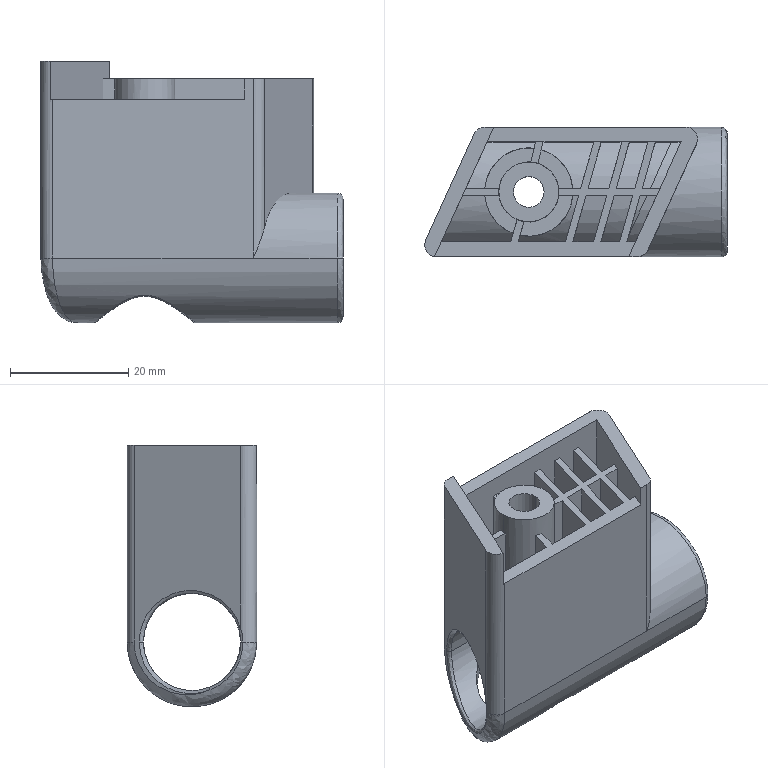Part | SolidWorks | features BaseBody 1 | 1 solid | 96 faces | box 51.079 x 21.892 x 44.191 mm | volume 16196 mm3 | plane 52 | cylinder 32 | spline 12 | commonest cylinder face diameters 21.394 x10 3.98 x4 14.926 x4 21.892 x4 5.174 x2 10.15 x2